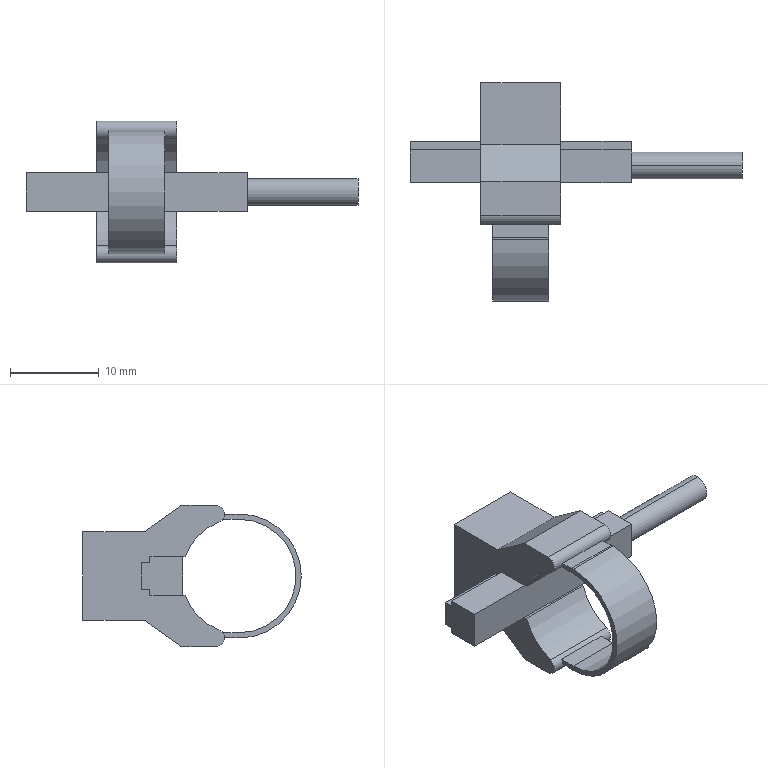Part | STEP file | 1 solid | 45 faces | box 37.5 x 24.7 x 16 mm | volume 1895 mm3 | plane 35 | cylinder 10 | commonest cylinder face diameters 14 x3 2 x2 3 x2 13 x2 12.8 x1